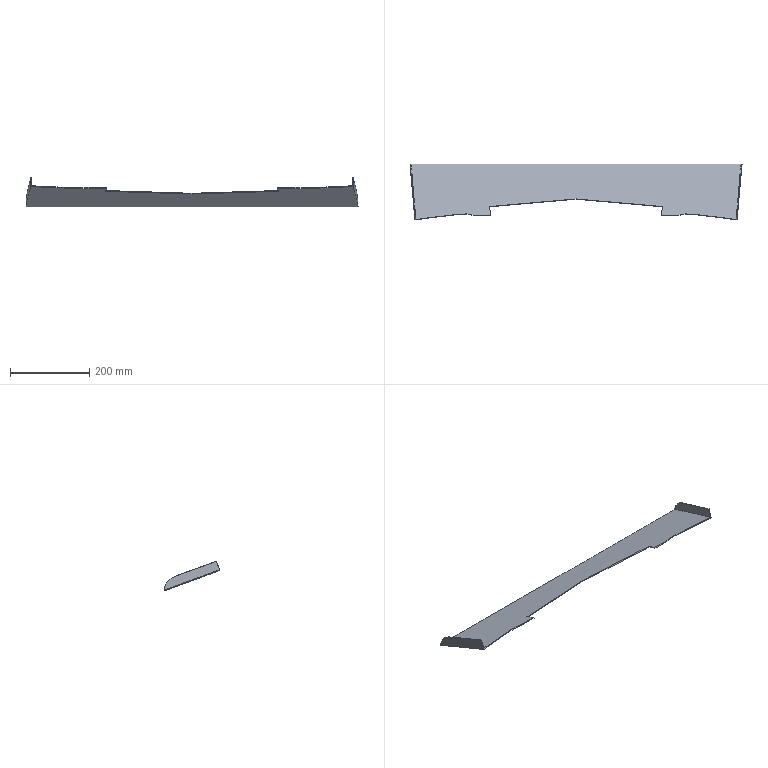Part | NX | features solid 2 | 1 solid | 21 faces | box 835.782 x 140.658 x 74.688 mm | volume 212187 mm3 | plane 17 | spline 2 | cylinder 2 | commonest cylinder face diameters 80 x2